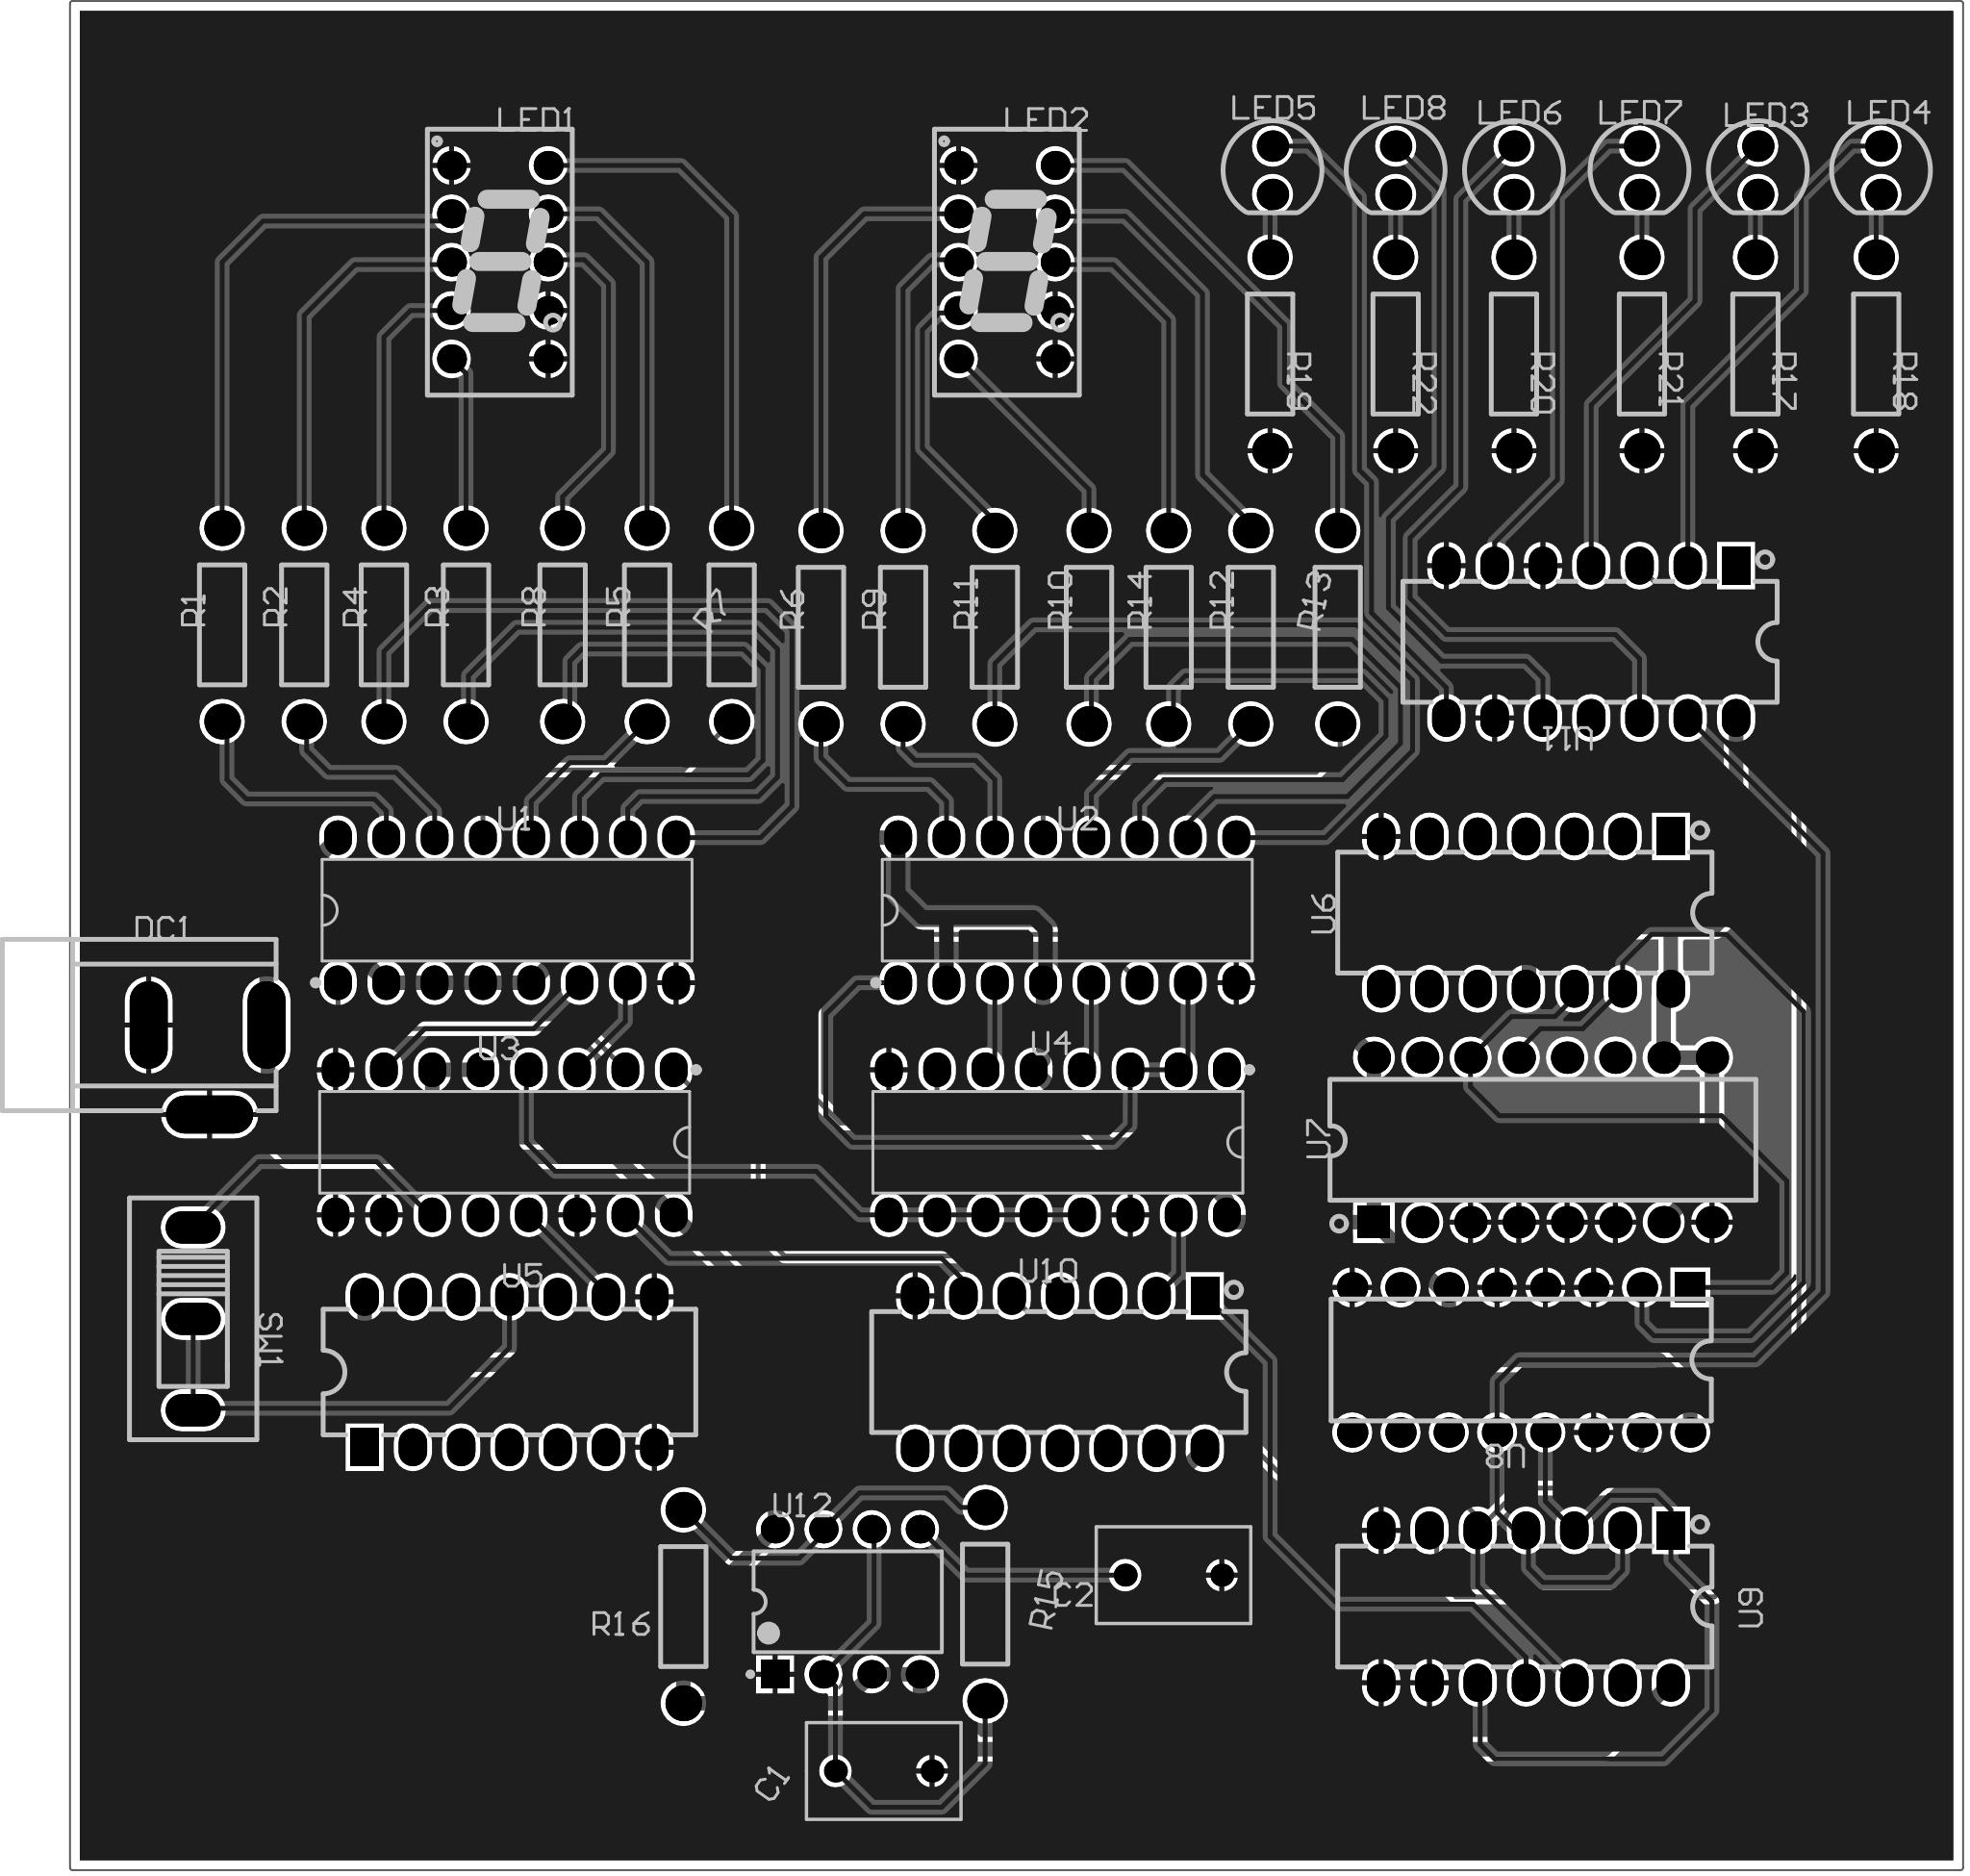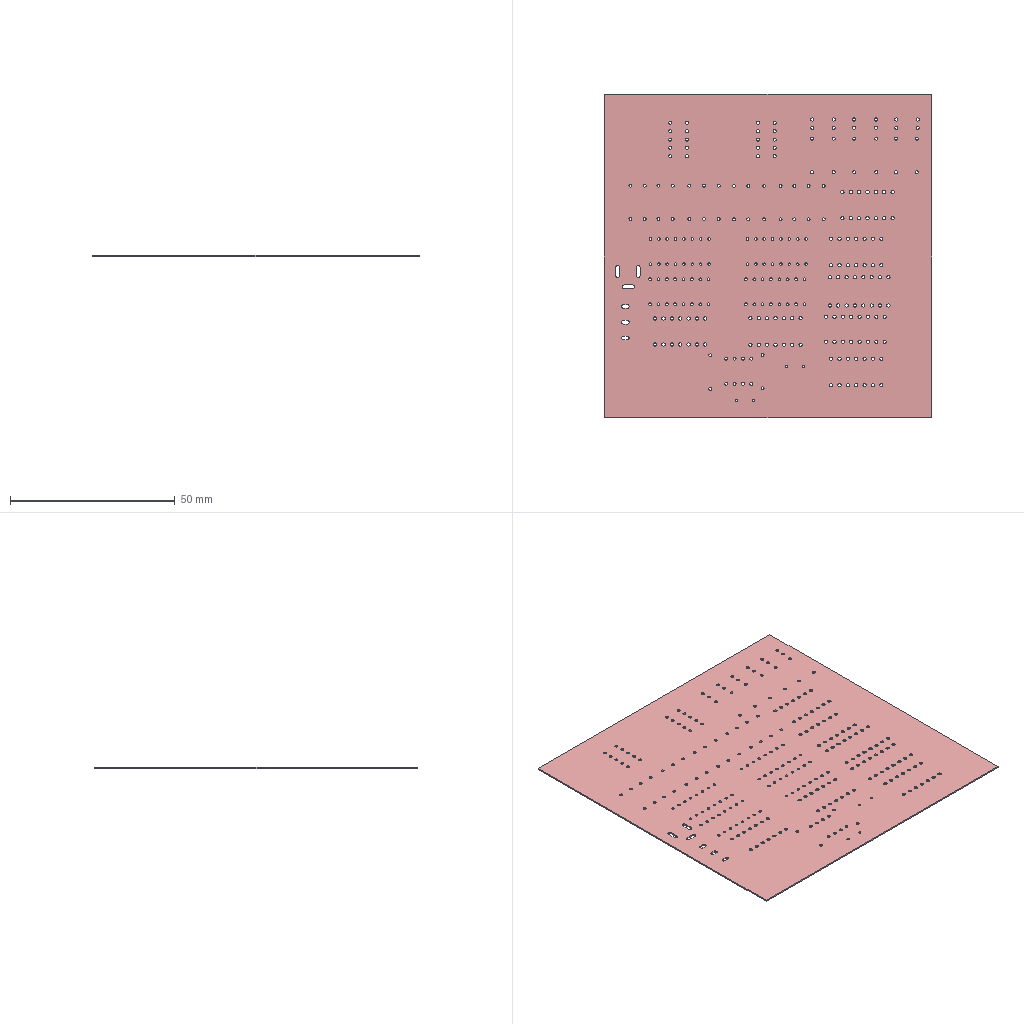Circuit board layout | Altium Designer | box 99.6 x 98.2 x 0.4 mm
Layer stack:
# Altium Designer layer stack of  (unit mm; dielectric type: 0 none, 1 core, 2 prepreg, 3 surface material)
index,name,kind,layer,copper_thickness_mm,dielectric_type,dielectric_thickness_mm,dielectric_material,dielectric_constant
0,Top Solder,dielectric,,,3,0.0102,Solder Resist,3.5
1,Top Paste,other,,,,,,
2,Top Overlay,other,,,,,,
3,Top Layer,copper,Top Layer,0.0356,,,,
4,Dielectric1,dielectric,,,0,0.32,FR-4,4.8
5,Bottom Layer,copper,Bottom Layer,0.0356,,,,
6,Bottom Overlay,other,,,,,,
7,Bottom Paste,other,,,,,,
8,Bottom Solder,dielectric,,,3,0.0102,Solder Resist,3.5
# drill layer pairs: low layer,high layer
drill_pair,Top Layer,Bottom Layer
Part placement:
Designator,Comment,Layer,Footprint,Center-X(mm),Center-Y(mm),Rotation
U12,100kHz,TopLayer,DIP-8_L9.8-W6.6-P2.54-LS7.6-BL,90.297,59.055,0
U8,XD74LS138,TopLayer,DIP-16_L19.8-W6.5-P2.54-LS7.6-BL,125.73,71.755,180
U7,SN74LS160N(LX),TopLayer,DIP-16_L22.4-W6.4-P2.54-LS8.64-BL,126.873,83.312,0
U11,SN74LS04N,TopLayer,PDIP-14_L19.7-W6.6-P2.54-LS8.3-BL,129.413,109.474,180
U10,SN74LS04N,TopLayer,PDIP-14_L19.7-W6.6-P2.54-LS8.3-BL,101.473,71.12,180
U9,SN74LS00N,TopLayer,PDIP-14_L19.7-W6.6-P2.54-LS8.3-BL,125.984,58.801,180
U6,SN74LS00N,TopLayer,PDIP-14_L19.7-W6.6-P2.54-LS8.3-BL,125.984,95.25,180
U5,SN74LS32N,TopLayer,PDIP-14_L19.6-W6.5-P2.54-LS7.9-BL,72.517,71.12,0
U4,XD74LS192,TopLayer,DIP-16_L19.3-W6.4-P2.54-LS7.6-BL,101.36,83.185,180
U3,XD74LS192,TopLayer,DIP-16_L19.3-W6.4-P2.54-LS7.6-BL,72.263,83.185,180
U2,XD74LS48,TopLayer,DIP-16_L19.3-W6.4-P2.54-LS7.6-BL,101.854,95.377,0
U1,XD74LS48,TopLayer,DIP-16_L19.3-W6.4-P2.54-LS7.6-BL,72.39,95.377,0
SW1,SS12D10G4 071,TopLayer,SW-TH_SHOU-HAN_SS12D10G4,55.88,73.914,270
R22,200,TopLayer,R_AXIAL-0.4,119.126,124.587,270
R21,200,TopLayer,R_AXIAL-0.4,132.08,124.587,270
R20,200,TopLayer,R_AXIAL-0.4,125.349,124.587,270
R19,200,TopLayer,R_AXIAL-0.4,112.522,124.587,270
R18,200,TopLayer,R_AXIAL-0.4,144.399,124.587,270
R17,200,TopLayer,R_AXIAL-0.4,138.049,124.587,270
R16,50K,TopLayer,R_AXIAL-0.4,81.661,58.801,90
R15,50K,TopLayer,R_AXIAL-0.4,97.536,58.928,270
R14,330,TopLayer,R_AXIAL-0.4,107.188,110.236,90
R13,330,TopLayer,R_AXIAL-0.4,116.078,110.236,90
R12,330,TopLayer,R_AXIAL-0.4,111.506,110.236,90
R11,330,TopLayer,R_AXIAL-0.4,98.044,110.236,90
R10,330,TopLayer,R_AXIAL-0.4,102.997,110.236,90
R9,330,TopLayer,R_AXIAL-0.4,93.218,110.236,90
R8,330,TopLayer,R_AXIAL-0.4,75.311,110.363,90
R7,330,TopLayer,R_AXIAL-0.4,84.201,110.363,90
R6,330,TopLayer,R_AXIAL-0.4,88.9,110.236,90
R5,330,TopLayer,R_AXIAL-0.4,79.756,110.363,90
R4,330,TopLayer,R_AXIAL-0.4,65.913,110.363,90
R3,330,TopLayer,R_AXIAL-0.4,70.231,110.363,90
R2,330,TopLayer,R_AXIAL-0.4,61.722,110.363,90
R1,330,TopLayer,R_AXIAL-0.4,57.404,110.363,90
LED8,LED-TH-5mm_R,TopLayer,LED-TH_BD5.0_RED,119.126,134.239,0
LED7,LED-TH-5mm_R,TopLayer,LED-TH_BD5.0_RED,131.953,134.239,0
LED6,LED-TH-5mm_R,TopLayer,LED-TH_BD5.0_RED,125.349,134.239,0
LED5,LED-TH-5mm_R,TopLayer,LED-TH_BD5.0_RED,112.649,134.239,0
LED4,LED-TH-5mm_R,TopLayer,LED-TH_BD5.0_RED,144.653,134.239,0
LED3,LED-TH-5mm_R,TopLayer,LED-TH_BD5.0_RED,138.176,134.239,0
LED2,FJ3161AH,TopLayer,LED-SEG-TH_10P-L14.0-W7.5-P2.54-S5.08-TL,98.679,129.413,0
LED1,FJ3161AH,TopLayer,LED-SEG-TH_10P-L14.0-W7.5-P2.54-S5.08-TL,72.009,129.413,0
DC1,DC005-2.0MM,TopLayer,DC-IN-TH_DC005,56.642,86.995,0
C2,10N,TopLayer,RAD-0.2,107.442,60.452,180
C1,10U,TopLayer,RAD-0.2,92.202,50.165,180
Pad and via stacks:
# Altium Designer via and pad stacks of  (unit mm). Each distinct definition once, with the count of objects using it.
# via: kind,start_layer,end_layer,hole_mm,diameter_mm,mode(0 simple;1 top-mid-bottom;2 full stack),diameter_per_layer,count,example_net
# pad: kind,layer,hole_mm,hole_type(0 round;1 square;2 slot),plating,top_size,top_shape(1 round;2 rect;3 octagon;9 rounded rect),mid_size,bottom_size,mode,footprint,size_per_layer,count,example
pad,Multi-Layer,0.9,0,plated,1.5x1.5,1,1.5x1.5,1.5x1.5,0,DIP-8_L9.8-W6.6-P2.54-LS7.6-BL,,7,U12.5
pad,Multi-Layer,0.9,0,plated,1.5x1.5,2,1.5x1.5,1.5x1.5,0,DIP-8_L9.8-W6.6-P2.54-LS7.6-BL,,1,U12.1
pad,Multi-Layer,1,0,plated,1.6x1.6,2,1.6x1.6,1.6x1.6,0,DIP-16_L19.8-W6.5-P2.54-LS7.6-BL,,1,U8.1
pad,Multi-Layer,1,0,plated,1.6x1.6,1,1.6x1.6,1.6x1.6,0,DIP-16_L19.8-W6.5-P2.54-LS7.6-BL,,15,U8.2
pad,Multi-Layer,1,0,plated,1.7x1.7,2,1.7x1.7,1.7x1.7,0,DIP-16_L22.4-W6.4-P2.54-LS8.64-BL,,1,U7.1
pad,Multi-Layer,1,0,plated,1.7x1.7,1,1.7x1.7,1.7x1.7,0,DIP-16_L22.4-W6.4-P2.54-LS8.64-BL,,15,U7.2
pad,Multi-Layer,1,0,plated,2x1.5,1,2x1.5,2x1.5,0,PDIP-14_L19.7-W6.6-P2.54-LS8.3-BL,,52,U11.8
pad,Multi-Layer,1,0,plated,2x1.5,2,2x1.5,2x1.5,0,PDIP-14_L19.7-W6.6-P2.54-LS8.3-BL,,4,U11.1
pad,Multi-Layer,1,0,plated,2x1.5,1,2x1.5,2x1.5,0,PDIP-14_L19.6-W6.5-P2.54-LS7.9-BL,,13,U5.8
pad,Multi-Layer,1,0,plated,2x1.5,2,2x1.5,2x1.5,0,PDIP-14_L19.6-W6.5-P2.54-LS7.9-BL,,1,U5.1
pad,Multi-Layer,0.8,0,plated,1.46x1.825,1,1.46x1.825,1.46x1.825,0,DIP-16_L19.3-W6.4-P2.54-LS7.6-BL,,64,U4.1
pad,Multi-Layer,1.1,2,plated,1.7x2.9,1,1.7x2.9,1.7x2.9,0,SW-TH_SHOU-HAN_SS12D10G4,,3,SW1.3
pad,Multi-Layer,0.8992,0,plated,1.88x1.88,1,1.88x1.88,1.88x1.88,0,R_AXIAL-0.4,,44,R22.2
pad,Multi-Layer,0.9652,0,plated,1.651x1.651,1,1.651x1.651,1.651x1.651,0,LED-TH_BD5.0_RED,,12,LED8.2
pad,Multi-Layer,0.9144,0,plated,1.524x1.524,1,1.524x1.524,1.524x1.524,0,LED-SEG-TH_10P-L14.0-W7.5-P2.54-S5.08-TL,,20,LED2.10
pad,Multi-Layer,1.2,2,plated,4.6x2,1,4.6x2,4.6x2,0,DC-IN-TH_DC005,,1,DC1.3
pad,Multi-Layer,1.2,2,plated,2x4.6,1,2x4.6,2x4.6,0,DC-IN-TH_DC005,,2,DC1.2
pad,Multi-Layer,0.7,0,plated,1.2x1.2,1,1.2x1.2,1.2x1.2,0,RAD-0.2,,4,C2.1
Copper pours:
name,layer,net,type(0 solid;1 hatched;2 none)
D,Bottom Layer,GND,0
D,Top Layer,GND,0
Design rules, without the lines most boards share:
# Altium Designer design rules of  (exported by Altium Designer, unit mm)
# columns: name | kind | enabled | priority | scope1 | scope2 | descriptor | typed fields (field=value)
SilkToSilkClearance | 55 | enabled | 1 | All | All | Silk to Silk (Clearance=0mil) (All),(All) |
SilkToSolderMaskClearance | 54 | enabled | 1 | IsPad | All | Silk To Solder Mask (Clearance=0mil) (IsPad),(All) |
MinimumSolderMaskSliver | 53 | enabled | 1 | All | All | Minimum Solder Mask Sliver (Gap=0mil) (All),(All) |
HoleToHoleClearance | 52 | enabled | 1 | All | All | Hole To Hole Clearance (Gap=10mil) (All),(All) | gap=0.254
DiffPairsRouting | 51 | enabled | 1 | All | All | Differential Pairs Uncoupled Length using the Gap Constraints (Min=10mil) (Max=10mil) (Prefered=10mil)  and Width Constraints (Min=15mil) (Max=15mil) (Prefered=15mil) (All) |
HoleSize | 42 | enabled | 1 | All | All | Hole Size Constraint (Min=1mil) (Max=6666mil) (All) |
SolderMaskExpansion | 13 | enabled | 1 | All | All | Solder Mask Expansion (Expansion =4mil) (All) | expansion=0.1016
PasteMaskExpansion | 14 | enabled | 1 | All | All | Paste Mask Expansion (Expansion =0mil) (All) | expansion=0
RoutingVias | 11 | enabled | 1 | All | All | Routing Via (MinHoleWidth=28mil) (MaxHoleWidth=28mil) (PreferredHoleWidth=28mil) (MinWidth=50mil) (MaxWidth=50mil) (PreferedWidth=50mil) (All) | via_min_hole=0.7112 via_max_hole=0.7112 via_preferred_diameter=1.27 via_preferred_hole=0.7112
Width | 2 | enabled | 1 | All | All | Width Constraint (Min=10mil) (Max=50mil) (Preferred=10mil) (All) |
PolygonConnect | 20 | enabled | 1 | All | All | Polygon Connect Rule(Relief Connect )(Conductor Width=10mil) (Relief Angle=90 Angle) (Entries=4) (Air Gap Width=10mil) (All),(All) | connect_style(0=relief,1=direct,2=none)=0 relief_conductor_width=0.254 relief_entries=4
PlaneConnect | 6 | enabled | 1 | All | All | Power Plane Connect Rule(Relief Connect )(Expansion=20mil) (Conductor Width=10mil) (Air Gap=10mil) (Entries=4) (All) | relief_conductor_width=0.254 relief_entries=4 relief_expansion=0.508
Clearance | 0 | enabled | 1 | All | All | Clearance Constraint (Gap=10mil) (All),(All) | gap=0.254